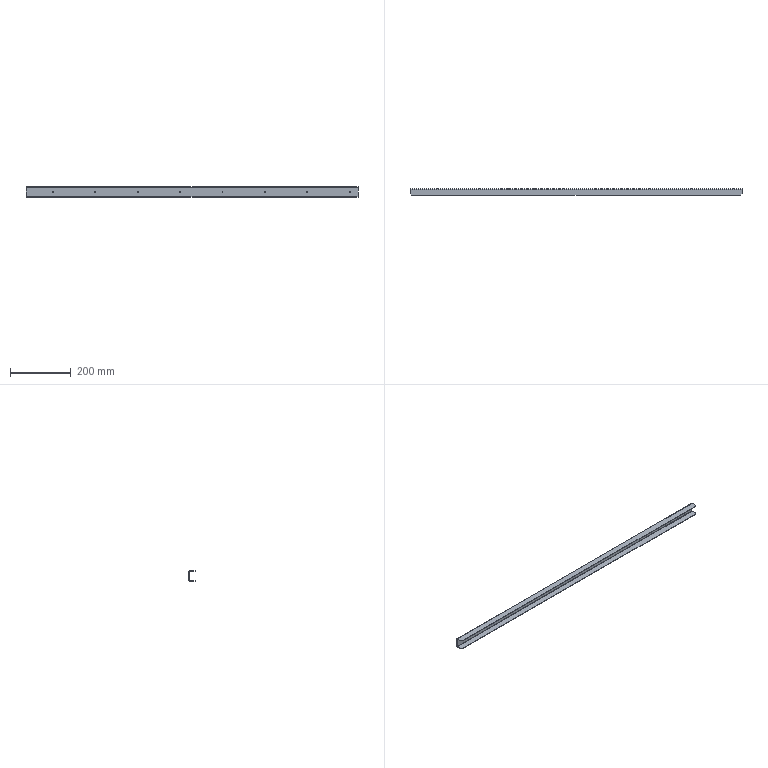Part | STEP file | b-013 | 1 solid | 42 faces | box 1094 x 21.5 x 33 mm | volume 117521 mm3 | plane 22 | cylinder 20 | commonest cylinder face diameters 3.3 x16 1.473 x2 4.473 x2